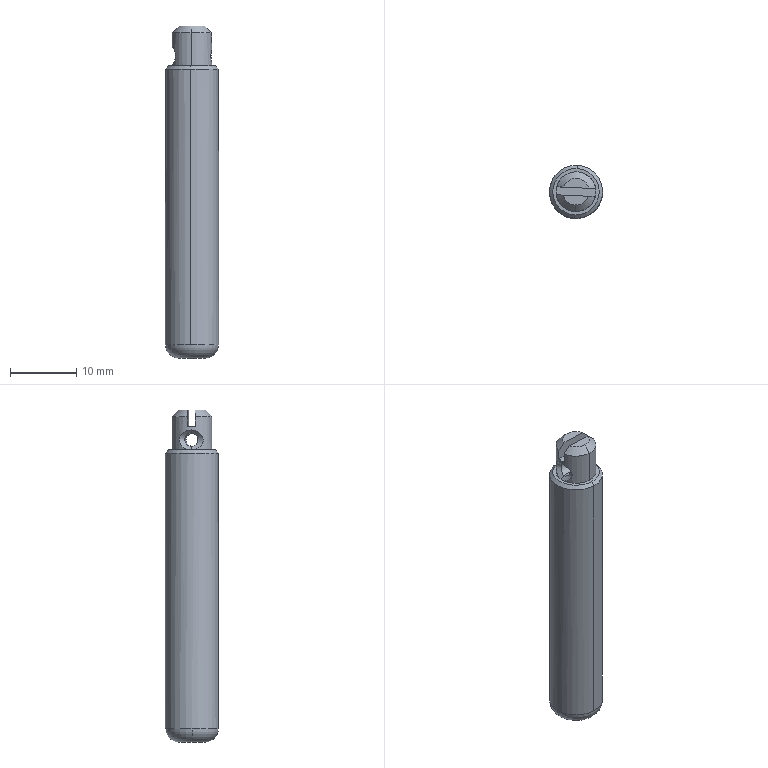Part | SolidWorks | features BaseBody 1 | 1 solid | 22 faces | box 8 x 8 x 50 mm | volume 2314 mm3 | plane 7 | cylinder 6 | cone 5 | spline 2 | torus 2 | commonest cylinder face diameters 2 x2 6 x2 8 x2
STEP:
#1=CARTESIAN_POINT('',(0.03983,28.012,-130.55));
#2=VERTEX_POINT('',#1);
#3=CARTESIAN_POINT('',(0.03996,28.015,-128.55));
#4=VERTEX_POINT('',#3);
#5=CARTESIAN_POINT('',(0.03983,28.012,-130.55));
#6=CARTESIAN_POINT('',(0.03364,27.875,-130.55));
#7=CARTESIAN_POINT('',(0.05576,27.735,-130.519));
#8=CARTESIAN_POINT('',(0.133,27.49,-130.414));
#9=CARTESIAN_POINT('',(0.187,27.383,-130.341));
#10=CARTESIAN_POINT('',(0.3031,27.204,-130.165));
#11=CARTESIAN_POINT('',(0.3627,27.129,-130.06));
#12=CARTESIAN_POINT('',(0.4571,27.024,-129.823));
#13=CARTESIAN_POINT('',(0.4923,26.992,-129.686));
#14=CARTESIAN_POINT('',(0.4912,26.993,-129.408));
#15=CARTESIAN_POINT('',(0.4562,27.025,-129.273));
#16=CARTESIAN_POINT('',(0.3609,27.132,-129.036));
#17=CARTESIAN_POINT('',(0.3014,27.205,-128.933));
#18=CARTESIAN_POINT('',(0.1856,27.386,-128.757));
#19=CARTESIAN_POINT('',(0.1323,27.492,-128.685));
#20=CARTESIAN_POINT('',(0.05554,27.737,-128.58));
#21=CARTESIAN_POINT('',(0.03327,27.875,-128.55));
#22=CARTESIAN_POINT('',(0.03996,28.015,-128.55));
#23=B_SPLINE_CURVE_WITH_KNOTS('',3,(#5,#6,#7,#8,#9,#10,#11,#12,#13,#14,#15,#16,#17,#18,#19,#20,#21,#22),.UNSPECIFIED.,.F.,.F.,(4,2,2,2,2,2,2,2,4),(0.003314,0.003727,0.00414,0.004553,0.004966,0.005379,0.005792,0.006205,0.006618),.UNSPECIFIED.);
#24=EDGE_CURVE('',#2,#4,#23,.T.);
#25=ORIENTED_EDGE('',*,*,#24,.F.);
#26=CARTESIAN_POINT('',(-0.4597,28.034,-131.05));
#27=VERTEX_POINT('',#26);
#28=CARTESIAN_POINT('',(0.03983,28.012,-130.55));
#29=CARTESIAN_POINT('',(-0.4597,28.034,-131.05));
#30=B_SPLINE_CURVE_WITH_KNOTS('',1,(#28,#29),.UNSPECIFIED.,.F.,.F.,(2,2),(0.009901,0.9896),.UNSPECIFIED.);
#31=EDGE_CURVE('',#2,#27,#30,.T.);
#32=ORIENTED_EDGE('',*,*,#31,.T.);
#33=CARTESIAN_POINT('',(-0.4595,28.039,-128.05));
#34=VERTEX_POINT('',#33);
#35=CARTESIAN_POINT('',(-0.4595,28.039,-128.05));
#36=CARTESIAN_POINT('',(-0.4701,27.815,-128.05));
#37=CARTESIAN_POINT('',(-0.4549,27.59,-128.084));
#38=CARTESIAN_POINT('',(-0.3813,27.169,-128.221));
#39=CARTESIAN_POINT('',(-0.3235,26.974,-128.322));
#40=CARTESIAN_POINT('',(-0.19,26.633,-128.58));
#41=CARTESIAN_POINT('',(-0.1141,26.487,-128.739));
#42=CARTESIAN_POINT('',(-0.02182,26.329,-129.02));
#43=CARTESIAN_POINT('',(0.005186,26.287,-129.121));
#44=CARTESIAN_POINT('',(0.0432,26.228,-129.331));
#45=CARTESIAN_POINT('',(0.05437,26.212,-129.443));
#46=CARTESIAN_POINT('',(0.05396,26.213,-129.664));
#47=CARTESIAN_POINT('',(0.04244,26.23,-129.775));
#48=CARTESIAN_POINT('',(0.003421,26.289,-129.986));
#49=CARTESIAN_POINT('',(-0.02341,26.332,-130.085));
#50=CARTESIAN_POINT('',(-0.1163,26.491,-130.366));
#51=CARTESIAN_POINT('',(-0.1903,26.633,-130.521));
#52=CARTESIAN_POINT('',(-0.3236,26.974,-130.778));
#53=CARTESIAN_POINT('',(-0.3805,27.166,-130.878));
#54=CARTESIAN_POINT('',(-0.4544,27.586,-131.015));
#55=CARTESIAN_POINT('',(-0.47,27.81,-131.05));
#56=CARTESIAN_POINT('',(-0.4597,28.034,-131.05));
#57=B_SPLINE_CURVE_WITH_KNOTS('',3,(#35,#36,#37,#38,#39,#40,#41,#42,#43,#44,#45,#46,#47,#48,#49,#50,#51,#52,#53,#54,#55,#56),.UNSPECIFIED.,.F.,.F.,(4,2,2,2,2,2,2,2,2,2,4),(0.005374,0.006046,0.006718,0.007391,0.007727,0.008063,0.008399,0.008735,0.009407,0.01008,0.01075),.UNSPECIFIED.);
#58=EDGE_CURVE('',#34,#27,#57,.T.);
#59=ORIENTED_EDGE('',*,*,#58,.F.);
#60=CARTESIAN_POINT('',(0.03996,28.015,-128.55));
#61=CARTESIAN_POINT('',(-0.4595,28.039,-128.05));
#62=B_SPLINE_CURVE_WITH_KNOTS('',1,(#60,#61),.UNSPECIFIED.,.F.,.F.,(2,2),(0.009901,0.9896),.UNSPECIFIED.);
#63=EDGE_CURVE('',#4,#34,#62,.T.);
#64=ORIENTED_EDGE('',*,*,#63,.F.);
#65=EDGE_LOOP('',(#25,#32,#59,#64));
#66=FACE_OUTER_BOUND('',#65,.T.);
#67=CARTESIAN_POINT('',(0.04501,28.015,-128.555));
#68=CARTESIAN_POINT('',(0.0577,28.283,-128.555));
#69=CARTESIAN_POINT('',(0.1783,28.533,-128.668));
#70=CARTESIAN_POINT('',(0.4502,28.877,-129.026));
#71=CARTESIAN_POINT('',(0.591,28.982,-129.281));
#72=CARTESIAN_POINT('',(0.5903,28.982,-129.822));
#73=CARTESIAN_POINT('',(0.4498,28.876,-130.075));
#74=CARTESIAN_POINT('',(0.1781,28.533,-130.432));
#75=CARTESIAN_POINT('',(0.05703,28.282,-130.546));
#76=CARTESIAN_POINT('',(0.03273,27.743,-130.544));
#77=CARTESIAN_POINT('',(0.1297,27.484,-130.43));
#78=CARTESIAN_POINT('',(0.3675,27.117,-130.072));
#79=CARTESIAN_POINT('',(0.4972,27.,-129.817));
#80=CARTESIAN_POINT('',(0.4952,27.001,-129.277));
#81=CARTESIAN_POINT('',(0.3667,27.119,-129.027));
#82=CARTESIAN_POINT('',(0.129,27.485,-128.669));
#83=CARTESIAN_POINT('',(0.03231,27.747,-128.555));
#84=CARTESIAN_POINT('',(0.04501,28.015,-128.555));
#85=CARTESIAN_POINT('',(-0.4595,28.039,-128.05));
#86=CARTESIAN_POINT('',(-0.4364,28.525,-128.05));
#87=CARTESIAN_POINT('',(-0.2839,28.983,-128.22));
#88=CARTESIAN_POINT('',(0.05333,29.613,-128.76));
#89=CARTESIAN_POINT('',(0.226,29.809,-129.144));
#90=CARTESIAN_POINT('',(0.225,29.808,-129.959));
#91=CARTESIAN_POINT('',(0.0529,29.613,-130.341));
#92=CARTESIAN_POINT('',(-0.2841,28.982,-130.88));
#93=CARTESIAN_POINT('',(-0.4372,28.523,-131.051));
#94=CARTESIAN_POINT('',(-0.4822,27.545,-131.049));
#95=CARTESIAN_POINT('',(-0.373,27.079,-130.877));
#96=CARTESIAN_POINT('',(-0.09732,26.421,-130.337));
#97=CARTESIAN_POINT('',(0.05533,26.211,-129.953));
#98=CARTESIAN_POINT('',(0.05298,26.214,-129.139));
#99=CARTESIAN_POINT('',(-0.09835,26.423,-128.761));
#100=CARTESIAN_POINT('',(-0.3738,27.081,-128.221));
#101=CARTESIAN_POINT('',(-0.4826,27.553,-128.05));
#102=CARTESIAN_POINT('',(-0.4595,28.039,-128.05));
#103=CARTESIAN_POINT('',(-0.4648,28.039,-128.045));
#104=CARTESIAN_POINT('',(-0.4416,28.528,-128.045));
#105=CARTESIAN_POINT('',(-0.2888,28.987,-128.216));
#106=CARTESIAN_POINT('',(0.04915,29.621,-128.757));
#107=CARTESIAN_POINT('',(0.2222,29.818,-129.143));
#108=CARTESIAN_POINT('',(0.2212,29.817,-129.961));
#109=CARTESIAN_POINT('',(0.04872,29.621,-130.344));
#110=CARTESIAN_POINT('',(-0.289,28.987,-130.885));
#111=CARTESIAN_POINT('',(-0.4425,28.525,-131.056));
#112=CARTESIAN_POINT('',(-0.4876,27.543,-131.054));
#113=CARTESIAN_POINT('',(-0.3783,27.074,-130.882));
#114=CARTESIAN_POINT('',(-0.1022,26.413,-130.34));
#115=CARTESIAN_POINT('',(0.05068,26.203,-129.954));
#116=CARTESIAN_POINT('',(0.04832,26.206,-129.138));
#117=CARTESIAN_POINT('',(-0.1033,26.416,-128.759));
#118=CARTESIAN_POINT('',(-0.3791,27.076,-128.216));
#119=CARTESIAN_POINT('',(-0.488,27.551,-128.045));
#120=CARTESIAN_POINT('',(-0.4648,28.039,-128.045));
#121=B_SPLINE_SURFACE_WITH_KNOTS('',1,3,((#67,#68,#69,#70,#71,#72,#73,#74,#75,#76,#77,#78,#79,#80,#81,#82,#83,#84),(#85,#86,#87,#88,#89,#90,#91,#92,#93,#94,#95,#96,#97,#98,#99,#100,#101,#102),(#103,#104,#105,#106,#107,#108,#109,#110,#111,#112,#113,#114,#115,#116,#117,#118,#119,#120)),.UNSPECIFIED.,.F.,.T.,.F.,(2,1,2),(4,2,2,2,2,2,2,2,4),(0.,0.9896,1.),(0.,0.125,0.25,0.375,0.5,0.625,0.75,0.875,1.),.UNSPECIFIED.);
#122=ADVANCED_FACE('',(#66),#121,.T.);
#123=CARTESIAN_POINT('',(2.347,23.901,-131.55));
#124=VERTEX_POINT('',#123);
#125=CARTESIAN_POINT('',(2.728,31.892,-131.55));
#126=VERTEX_POINT('',#125);
#127=CARTESIAN_POINT('',(2.537,27.896,-131.55));
#128=DIRECTION('',(0.,0.,-1.));
#129=DIRECTION('',(0.0476,0.9989,0.));
#130=AXIS2_PLACEMENT_3D('',#127,#128,#129);
#131=CIRCLE('',#130,4.);
#132=EDGE_CURVE('',#124,#126,#131,.T.);
#133=ORIENTED_EDGE('',*,*,#132,.T.);
#134=CARTESIAN_POINT('',(2.728,31.892,-173.05));
#135=VERTEX_POINT('',#134);
#136=CARTESIAN_POINT('',(2.728,31.892,-125.05));
#137=DIRECTION('',(0.,0.,-1.));
#138=VECTOR('',#137,1000.);
#139=LINE('',#136,#138);
#140=EDGE_CURVE('',#126,#135,#139,.T.);
#141=ORIENTED_EDGE('',*,*,#140,.T.);
#142=CARTESIAN_POINT('',(-1.463,27.896,-173.05));
#143=VERTEX_POINT('',#142);
#144=CARTESIAN_POINT('',(2.537,27.896,-173.05));
#145=DIRECTION('',(0.,0.,1.));
#146=DIRECTION('',(0.0476,0.9989,0.));
#147=AXIS2_PLACEMENT_3D('',#144,#145,#146);
#148=CIRCLE('',#147,4.);
#149=EDGE_CURVE('',#135,#143,#148,.T.);
#150=ORIENTED_EDGE('',*,*,#149,.T.);
#151=CARTESIAN_POINT('',(2.347,23.901,-173.05));
#152=VERTEX_POINT('',#151);
#153=CARTESIAN_POINT('',(2.537,27.896,-173.05));
#154=DIRECTION('',(0.,0.,1.));
#155=DIRECTION('',(0.0476,0.9989,0.));
#156=AXIS2_PLACEMENT_3D('',#153,#154,#155);
#157=CIRCLE('',#156,4.);
#158=EDGE_CURVE('',#143,#152,#157,.T.);
#159=ORIENTED_EDGE('',*,*,#158,.T.);
#160=CARTESIAN_POINT('',(2.347,23.901,-125.05));
#161=DIRECTION('',(0.,0.,-1.));
#162=VECTOR('',#161,1000.);
#163=LINE('',#160,#162);
#164=EDGE_CURVE('',#124,#152,#163,.T.);
#165=ORIENTED_EDGE('',*,*,#164,.F.);
#166=EDGE_LOOP('',(#133,#141,#150,#159,#165));
#167=FACE_OUTER_BOUND('',#166,.T.);
#168=CARTESIAN_POINT('',(2.537,27.896,-125.05));
#169=DIRECTION('',(0.,0.,-1.));
#170=DIRECTION('',(-0.0476,-0.9989,0.));
#171=AXIS2_PLACEMENT_3D('',#168,#169,#170);
#172=CYLINDRICAL_SURFACE('',#171,4.);
#173=ADVANCED_FACE('',(#167),#172,.T.);
#174=CARTESIAN_POINT('',(-0.4595,28.039,-131.05));
#175=VERTEX_POINT('',#174);
#176=CARTESIAN_POINT('',(2.394,24.9,-131.05));
#177=VERTEX_POINT('',#176);
#178=CARTESIAN_POINT('',(2.537,27.896,-131.05));
#179=DIRECTION('',(0.,0.,1.));
#180=DIRECTION('',(0.0476,0.9989,0.));
#181=AXIS2_PLACEMENT_3D('',#178,#179,#180);
#182=CIRCLE('',#181,3.);
#183=EDGE_CURVE('',#175,#177,#182,.T.);
#184=ORIENTED_EDGE('',*,*,#183,.T.);
#185=CARTESIAN_POINT('',(2.394,24.9,-126.05));
#186=VERTEX_POINT('',#185);
#187=CARTESIAN_POINT('',(2.394,24.9,-131.05));
#188=DIRECTION('',(0.,0.,1.));
#189=VECTOR('',#188,1000.);
#190=LINE('',#187,#189);
#191=EDGE_CURVE('',#177,#186,#190,.T.);
#192=ORIENTED_EDGE('',*,*,#191,.T.);
#193=CARTESIAN_POINT('',(-0.4275,27.437,-126.05));
#194=VERTEX_POINT('',#193);
#195=CARTESIAN_POINT('',(2.537,27.896,-126.05));
#196=DIRECTION('',(0.,0.,-1.));
#197=DIRECTION('',(0.0476,0.9989,0.));
#198=AXIS2_PLACEMENT_3D('',#195,#196,#197);
#199=CIRCLE('',#198,3.);
#200=EDGE_CURVE('',#186,#194,#199,.T.);
#201=ORIENTED_EDGE('',*,*,#200,.T.);
#202=CARTESIAN_POINT('',(-0.4275,27.437,-127.55));
#203=VERTEX_POINT('',#202);
#204=CARTESIAN_POINT('',(-0.4275,27.437,-127.55));
#205=DIRECTION('',(0.,0.,-1.));
#206=VECTOR('',#205,1000.);
#207=LINE('',#204,#206);
#208=EDGE_CURVE('',#194,#203,#207,.T.);
#209=ORIENTED_EDGE('',*,*,#208,.T.);
#210=CARTESIAN_POINT('',(-0.3704,28.635,-127.55));
#211=VERTEX_POINT('',#210);
#212=CARTESIAN_POINT('',(2.537,27.896,-127.55));
#213=DIRECTION('',(0.,0.,1.));
#214=DIRECTION('',(0.0476,0.9989,0.));
#215=AXIS2_PLACEMENT_3D('',#212,#213,#214);
#216=CIRCLE('',#215,3.);
#217=EDGE_CURVE('',#211,#203,#216,.T.);
#218=ORIENTED_EDGE('',*,*,#217,.F.);
#219=CARTESIAN_POINT('',(-0.3704,28.635,-126.05));
#220=VERTEX_POINT('',#219);
#221=CARTESIAN_POINT('',(-0.3704,28.635,-127.55));
#222=DIRECTION('',(0.,0.,-1.));
#223=VECTOR('',#222,1000.);
#224=LINE('',#221,#223);
#225=EDGE_CURVE('',#220,#211,#224,.T.);
#226=ORIENTED_EDGE('',*,*,#225,.F.);
#227=CARTESIAN_POINT('',(2.68,30.893,-126.05));
#228=VERTEX_POINT('',#227);
#229=CARTESIAN_POINT('',(2.537,27.896,-126.05));
#230=DIRECTION('',(0.,0.,-1.));
#231=DIRECTION('',(0.0476,0.9989,0.));
#232=AXIS2_PLACEMENT_3D('',#229,#230,#231);
#233=CIRCLE('',#232,3.);
#234=EDGE_CURVE('',#220,#228,#233,.T.);
#235=ORIENTED_EDGE('',*,*,#234,.T.);
#236=CARTESIAN_POINT('',(2.68,30.893,-131.05));
#237=VERTEX_POINT('',#236);
#238=CARTESIAN_POINT('',(2.68,30.893,-131.05));
#239=DIRECTION('',(0.,0.,1.));
#240=VECTOR('',#239,1000.);
#241=LINE('',#238,#240);
#242=EDGE_CURVE('',#237,#228,#241,.T.);
#243=ORIENTED_EDGE('',*,*,#242,.F.);
#244=CARTESIAN_POINT('',(2.537,27.896,-131.05));
#245=DIRECTION('',(0.,0.,1.));
#246=DIRECTION('',(0.0476,0.9989,0.));
#247=AXIS2_PLACEMENT_3D('',#244,#245,#246);
#248=CIRCLE('',#247,3.);
#249=EDGE_CURVE('',#237,#175,#248,.T.);
#250=ORIENTED_EDGE('',*,*,#249,.T.);
#251=CARTESIAN_POINT('',(-0.4595,28.039,-131.05));
#252=CARTESIAN_POINT('',(-0.4488,28.263,-131.05));
#253=CARTESIAN_POINT('',(-0.4123,28.485,-131.016));
#254=CARTESIAN_POINT('',(-0.2992,28.896,-130.879));
#255=CARTESIAN_POINT('',(-0.2232,29.085,-130.778));
#256=CARTESIAN_POINT('',(-0.05789,29.413,-130.521));
#257=CARTESIAN_POINT('',(0.03136,29.55,-130.362));
#258=CARTESIAN_POINT('',(0.1384,29.699,-130.081));
#259=CARTESIAN_POINT('',(0.1692,29.738,-129.981));
#260=CARTESIAN_POINT('',(0.2128,29.793,-129.771));
#261=CARTESIAN_POINT('',(0.2257,29.809,-129.659));
#262=CARTESIAN_POINT('',(0.2254,29.808,-129.437));
#263=CARTESIAN_POINT('',(0.2122,29.793,-129.325));
#264=CARTESIAN_POINT('',(0.1677,29.737,-129.115));
#265=CARTESIAN_POINT('',(0.1363,29.696,-129.014));
#266=CARTESIAN_POINT('',(0.02984,29.548,-128.736));
#267=CARTESIAN_POINT('',(-0.05896,29.411,-128.577));
#268=CARTESIAN_POINT('',(-0.2241,29.083,-128.32));
#269=CARTESIAN_POINT('',(-0.2992,28.897,-128.221));
#270=CARTESIAN_POINT('',(-0.4122,28.485,-128.084));
#271=CARTESIAN_POINT('',(-0.4488,28.263,-128.05));
#272=CARTESIAN_POINT('',(-0.4595,28.039,-128.05));
#273=B_SPLINE_CURVE_WITH_KNOTS('',3,(#251,#252,#253,#254,#255,#256,#257,#258,#259,#260,#261,#262,#263,#264,#265,#266,#267,#268,#269,#270,#271,#272),.UNSPECIFIED.,.F.,.F.,(4,2,2,2,2,2,2,2,2,2,4),(0.,0.0006718,0.001344,0.002015,0.002351,0.002687,0.003023,0.003359,0.004031,0.004702,0.005374),.UNSPECIFIED.);
#274=EDGE_CURVE('',#175,#34,#273,.T.);
#275=ORIENTED_EDGE('',*,*,#274,.T.);
#276=ORIENTED_EDGE('',*,*,#58,.T.);
#277=CARTESIAN_POINT('',(-0.4597,28.034,-131.05));
#278=CARTESIAN_POINT('',(-0.4597,28.035,-131.05));
#279=CARTESIAN_POINT('',(-0.4596,28.036,-131.05));
#280=CARTESIAN_POINT('',(-0.4596,28.037,-131.05));
#281=CARTESIAN_POINT('',(-0.4595,28.038,-131.05));
#282=CARTESIAN_POINT('',(-0.4595,28.039,-131.05));
#283=B_SPLINE_CURVE_WITH_KNOTS('',3,(#277,#278,#279,#280,#281,#282),.UNSPECIFIED.,.F.,.F.,(4,2,4),(0.01075,0.01075,0.01076),.UNSPECIFIED.);
#284=EDGE_CURVE('',#27,#175,#283,.T.);
#285=ORIENTED_EDGE('',*,*,#284,.T.);
#286=EDGE_LOOP('',(#184,#192,#201,#209,#218,#226,#235,#243,#250,#275,#276,#285));
#287=FACE_OUTER_BOUND('',#286,.T.);
#288=CARTESIAN_POINT('',(2.537,27.896,-131.05));
#289=DIRECTION('',(0.,0.,1.));
#290=DIRECTION('',(0.0476,0.9989,0.));
#291=AXIS2_PLACEMENT_3D('',#288,#289,#290);
#292=CYLINDRICAL_SURFACE('',#291,3.);
#293=ADVANCED_FACE('',(#287),#292,.T.);
#294=CARTESIAN_POINT('',(5.534,27.753,-128.55));
#295=VERTEX_POINT('',#294);
#296=CARTESIAN_POINT('',(5.534,27.753,-130.55));
#297=VERTEX_POINT('',#296);
#298=CARTESIAN_POINT('',(5.534,27.753,-128.55));
#299=CARTESIAN_POINT('',(5.527,27.62,-128.55));
#300=CARTESIAN_POINT('',(5.512,27.49,-128.577));
#301=CARTESIAN_POINT('',(5.469,27.25,-128.677));
#302=CARTESIAN_POINT('',(5.442,27.141,-128.751));
#303=CARTESIAN_POINT('',(5.389,26.961,-128.935));
#304=CARTESIAN_POINT('',(5.363,26.887,-129.045));
#305=CARTESIAN_POINT('',(5.326,26.789,-129.286));
#306=CARTESIAN_POINT('',(5.315,26.763,-129.418));
#307=CARTESIAN_POINT('',(5.315,26.763,-129.682));
#308=CARTESIAN_POINT('',(5.326,26.788,-129.813));
#309=CARTESIAN_POINT('',(5.363,26.888,-130.056));
#310=CARTESIAN_POINT('',(5.389,26.96,-130.165));
#311=CARTESIAN_POINT('',(5.442,27.142,-130.349));
#312=CARTESIAN_POINT('',(5.469,27.251,-130.423));
#313=CARTESIAN_POINT('',(5.512,27.491,-130.523));
#314=CARTESIAN_POINT('',(5.527,27.622,-130.55));
#315=CARTESIAN_POINT('',(5.534,27.753,-130.55));
#316=B_SPLINE_CURVE_WITH_KNOTS('',3,(#298,#299,#300,#301,#302,#303,#304,#305,#306,#307,#308,#309,#310,#311,#312,#313,#314,#315),.UNSPECIFIED.,.F.,.F.,(4,2,2,2,2,2,2,2,4),(0.,0.0003936,0.0007871,0.001181,0.001574,0.001968,0.002361,0.002755,0.003149),.UNSPECIFIED.);
#317=EDGE_CURVE('',#295,#297,#316,.T.);
#318=ORIENTED_EDGE('',*,*,#317,.T.);
#319=CARTESIAN_POINT('',(0.03996,28.015,-130.55));
#320=VERTEX_POINT('',#319);
#321=CARTESIAN_POINT('',(10.528,27.515,-130.55));
#322=DIRECTION('',(-0.9989,0.0476,0.));
#323=VECTOR('',#322,1000.);
#324=LINE('',#321,#323);
#325=EDGE_CURVE('',#297,#320,#324,.T.);
#326=ORIENTED_EDGE('',*,*,#325,.T.);
#327=CARTESIAN_POINT('',(0.03996,28.015,-130.55));
#328=CARTESIAN_POINT('',(0.03994,28.015,-130.55));
#329=CARTESIAN_POINT('',(0.03989,28.014,-130.55));
#330=CARTESIAN_POINT('',(0.03985,28.013,-130.55));
#331=CARTESIAN_POINT('',(0.03983,28.012,-130.55));
#332=B_SPLINE_CURVE_WITH_KNOTS('',3,(#327,#328,#329,#330,#331),.UNSPECIFIED.,.F.,.F.,(4,1,4),(0.003311,0.003313,0.003314),.UNSPECIFIED.);
#333=EDGE_CURVE('',#320,#2,#332,.T.);
#334=ORIENTED_EDGE('',*,*,#333,.T.);
#335=ORIENTED_EDGE('',*,*,#24,.T.);
#336=CARTESIAN_POINT('',(10.528,27.515,-128.55));
#337=DIRECTION('',(-0.9989,0.0476,0.));
#338=VECTOR('',#337,1000.);
#339=LINE('',#336,#338);
#340=EDGE_CURVE('',#295,#4,#339,.T.);
#341=ORIENTED_EDGE('',*,*,#340,.F.);
#342=EDGE_LOOP('',(#318,#326,#334,#335,#341));
#343=FACE_OUTER_BOUND('',#342,.T.);
#344=CARTESIAN_POINT('',(10.528,27.515,-129.55));
#345=DIRECTION('',(-0.9989,0.0476,0.));
#346=DIRECTION('',(0.,0.,1.));
#347=AXIS2_PLACEMENT_3D('',#344,#345,#346);
#348=CYLINDRICAL_SURFACE('',#347,1.);
#349=ADVANCED_FACE('',(#343),#348,.F.);
#350=CARTESIAN_POINT('',(2.442,25.898,-125.05));
#351=VERTEX_POINT('',#350);
#352=CARTESIAN_POINT('',(4.414,27.206,-125.05));
#353=VERTEX_POINT('',#352);
#354=CARTESIAN_POINT('',(2.537,27.896,-125.05));
#355=DIRECTION('',(0.,0.,1.));
#356=DIRECTION('',(0.0476,0.9989,0.));
#357=AXIS2_PLACEMENT_3D('',#354,#355,#356);
#358=CIRCLE('',#357,2.);
#359=EDGE_CURVE('',#351,#353,#358,.T.);
#360=ORIENTED_EDGE('',*,*,#359,.F.);
#361=CARTESIAN_POINT('',(2.442,25.898,-125.05));
#362=DIRECTION('',(-0.03366,-0.7063,-0.7071));
#363=VECTOR('',#362,1000.);
#364=LINE('',#361,#363);
#365=EDGE_CURVE('',#351,#186,#364,.T.);
#366=ORIENTED_EDGE('',*,*,#365,.T.);
#367=CARTESIAN_POINT('',(5.445,27.157,-126.05));
#368=VERTEX_POINT('',#367);
#369=CARTESIAN_POINT('',(2.537,27.896,-126.05));
#370=DIRECTION('',(0.,0.,-1.));
#371=DIRECTION('',(0.0476,0.9989,0.));
#372=AXIS2_PLACEMENT_3D('',#369,#370,#371);
#373=CIRCLE('',#372,3.);
#374=EDGE_CURVE('',#368,#186,#373,.T.);
#375=ORIENTED_EDGE('',*,*,#374,.F.);
#376=CARTESIAN_POINT('',(4.414,27.206,-125.05));
#377=CARTESIAN_POINT('',(4.76,27.19,-125.381));
#378=CARTESIAN_POINT('',(5.103,27.173,-125.715));
#379=CARTESIAN_POINT('',(5.445,27.157,-126.05));
#380=B_SPLINE_CURVE_WITH_KNOTS('',3,(#376,#377,#378,#379),.UNSPECIFIED.,.F.,.F.,(4,4),(0.,0.001437),.UNSPECIFIED.);
#381=EDGE_CURVE('',#353,#368,#380,.T.);
#382=ORIENTED_EDGE('',*,*,#381,.F.);
#383=EDGE_LOOP('',(#360,#366,#375,#382));
#384=FACE_OUTER_BOUND('',#383,.T.);
#385=CARTESIAN_POINT('',(2.537,27.896,-125.05));
#386=DIRECTION('',(0.,0.,-1.));
#387=DIRECTION('',(-0.0476,-0.9989,0.));
#388=AXIS2_PLACEMENT_3D('',#385,#386,#387);
#389=CONICAL_SURFACE('',#388,2.,0.7854);
#390=ADVANCED_FACE('',(#384),#389,.T.);
#391=CARTESIAN_POINT('',(2.704,31.392,-131.05));
#392=VERTEX_POINT('',#391);
#393=CARTESIAN_POINT('',(2.371,24.4,-131.05));
#394=VERTEX_POINT('',#393);
#395=CARTESIAN_POINT('',(2.537,27.896,-131.05));
#396=DIRECTION('',(0.,0.,1.));
#397=DIRECTION('',(0.0476,0.9989,0.));
#398=AXIS2_PLACEMENT_3D('',#395,#396,#397);
#399=CIRCLE('',#398,3.5);
#400=EDGE_CURVE('',#392,#394,#399,.T.);
#401=ORIENTED_EDGE('',*,*,#400,.F.);
#402=CARTESIAN_POINT('',(2.704,31.392,-131.05));
#403=DIRECTION('',(0.03366,0.7063,-0.7071));
#404=VECTOR('',#403,1000.);
#405=LINE('',#402,#404);
#406=EDGE_CURVE('',#392,#126,#405,.T.);
#407=ORIENTED_EDGE('',*,*,#406,.T.);
#408=ORIENTED_EDGE('',*,*,#132,.F.);
#409=CARTESIAN_POINT('',(2.371,24.4,-131.05));
#410=DIRECTION('',(-0.03366,-0.7063,-0.7071));
#411=VECTOR('',#410,1000.);
#412=LINE('',#409,#411);
#413=EDGE_CURVE('',#394,#124,#412,.T.);
#414=ORIENTED_EDGE('',*,*,#413,.F.);
#415=EDGE_LOOP('',(#401,#407,#408,#414));
#416=FACE_OUTER_BOUND('',#415,.T.);
#417=CARTESIAN_POINT('',(2.537,27.896,-131.05));
#418=DIRECTION('',(0.,0.,-1.));
#419=DIRECTION('',(-0.0476,-0.9989,0.));
#420=AXIS2_PLACEMENT_3D('',#417,#418,#419);
#421=CONICAL_SURFACE('',#420,3.5,0.7854);
#422=ADVANCED_FACE('',(#416),#421,.T.);
#423=CARTESIAN_POINT('',(4.537,27.896,-175.05));
#424=VERTEX_POINT('',#423);
#425=CARTESIAN_POINT('',(0.5371,27.896,-175.05));
#426=VERTEX_POINT('',#425);
#427=CARTESIAN_POINT('',(2.537,27.896,-175.05));
#428=DIRECTION('',(0.,0.,-1.));
#429=DIRECTION('',(0.0476,0.9989,0.));
#430=AXIS2_PLACEMENT_3D('',#427,#428,#429);
#431=CIRCLE('',#430,2.);
#432=EDGE_CURVE('',#424,#426,#431,.T.);
#433=ORIENTED_EDGE('',*,*,#432,.F.);
#434=CARTESIAN_POINT('',(6.537,27.896,-173.05));
#435=VERTEX_POINT('',#434);
#436=CARTESIAN_POINT('',(4.537,27.896,-173.05));
#437=DIRECTION('',(0.,-1.,0.));
#438=DIRECTION('',(1.,0.,0.));
#439=AXIS2_PLACEMENT_3D('',#436,#437,#438);
#440=CIRCLE('',#439,2.);
#441=EDGE_CURVE('',#424,#435,#440,.T.);
#442=ORIENTED_EDGE('',*,*,#441,.T.);
#443=CARTESIAN_POINT('',(2.537,27.896,-173.05));
#444=DIRECTION('',(0.,0.,1.));
#445=DIRECTION('',(0.0476,0.9989,0.));
#446=AXIS2_PLACEMENT_3D('',#443,#444,#445);
#447=CIRCLE('',#446,4.);
#448=EDGE_CURVE('',#152,#435,#447,.T.);
#449=ORIENTED_EDGE('',*,*,#448,.F.);
#450=ORIENTED_EDGE('',*,*,#158,.F.);
#451=CARTESIAN_POINT('',(0.5371,27.896,-173.05));
#452=DIRECTION('',(0.,1.,0.));
#453=DIRECTION('',(0.,0.,1.));
#454=AXIS2_PLACEMENT_3D('',#451,#452,#453);
#455=CIRCLE('',#454,2.);
#456=EDGE_CURVE('',#426,#143,#455,.T.);
#457=ORIENTED_EDGE('',*,*,#456,.F.);
#458=EDGE_LOOP('',(#433,#442,#449,#450,#457));
#459=FACE_OUTER_BOUND('',#458,.T.);
#460=CARTESIAN_POINT('',(2.537,27.896,-173.05));
#461=DIRECTION('',(0.,0.,1.));
#462=DIRECTION('',(-1.,0.,0.));
#463=AXIS2_PLACEMENT_3D('',#460,#461,#462);
#464=TOROIDAL_SURFACE('',#463,2.,2.);
#465=ADVANCED_FACE('',(#459),#464,.T.);
#466=ORIENTED_EDGE('',*,*,#441,.F.);
#467=CARTESIAN_POINT('',(2.537,27.896,-175.05));
#468=DIRECTION('',(0.,0.,-1.));
#469=DIRECTION('',(0.0476,0.9989,0.));
#470=AXIS2_PLACEMENT_3D('',#467,#468,#469);
#471=CIRCLE('',#470,2.);
#472=EDGE_CURVE('',#426,#424,#471,.T.);
#473=ORIENTED_EDGE('',*,*,#472,.F.);
#474=ORIENTED_EDGE('',*,*,#456,.T.);
#475=ORIENTED_EDGE('',*,*,#149,.F.);
#476=CARTESIAN_POINT('',(2.537,27.896,-173.05));
#477=DIRECTION('',(0.,0.,1.));
#478=DIRECTION('',(0.0476,0.9989,0.));
#479=AXIS2_PLACEMENT_3D('',#476,#477,#478);
#480=CIRCLE('',#479,4.);
#481=EDGE_CURVE('',#435,#135,#480,.T.);
#482=ORIENTED_EDGE('',*,*,#481,.F.);
#483=EDGE_LOOP('',(#466,#473,#474,#475,#482));
#484=FACE_OUTER_BOUND('',#483,.T.);
#485=CARTESIAN_POINT('',(2.537,27.896,-173.05));
#486=DIRECTION('',(0.,0.,1.));
#487=DIRECTION('',(-1.,0.,0.));
#488=AXIS2_PLACEMENT_3D('',#485,#486,#487);
#489=TOROIDAL_SURFACE('',#488,2.,2.);
#490=ADVANCED_FACE('',(#484),#489,.T.);
#491=ORIENTED_EDGE('',*,*,#406,.F.);
#492=CARTESIAN_POINT('',(2.537,27.896,-131.05));
#493=DIRECTION('',(0.,0.,1.));
#494=DIRECTION('',(0.0476,0.9989,0.));
#495=AXIS2_PLACEMENT_3D('',#492,#493,#494);
#496=CIRCLE('',#495,3.5);
#497=EDGE_CURVE('',#394,#392,#496,.T.);
#498=ORIENTED_EDGE('',*,*,#497,.F.);
#499=ORIENTED_EDGE('',*,*,#413,.T.);
#500=CARTESIAN_POINT('',(2.537,27.896,-131.55));
#501=DIRECTION('',(0.,0.,-1.));
#502=DIRECTION('',(0.0476,0.9989,0.));
#503=AXIS2_PLACEMENT_3D('',#500,#501,#502);
#504=CIRCLE('',#503,4.);
#505=EDGE_CURVE('',#126,#124,#504,.T.);
#506=ORIENTED_EDGE('',*,*,#505,.F.);
#507=EDGE_LOOP('',(#491,#498,#499,#506));
#508=FACE_OUTER_BOUND('',#507,.T.);
#509=CARTESIAN_POINT('',(2.537,27.896,-131.05));
#510=DIRECTION('',(0.,0.,-1.));
#511=DIRECTION('',(-0.0476,-0.9989,0.));
#512=AXIS2_PLACEMENT_3D('',#509,#510,#511);
#513=CONICAL_SURFACE('',#512,3.5,0.7854);
#514=ADVANCED_FACE('',(#508),#513,.T.);
#515=ORIENTED_EDGE('',*,*,#365,.F.);
#516=CARTESIAN_POINT('',(0.6028,27.388,-125.05));
#517=VERTEX_POINT('',#516);
#518=CARTESIAN_POINT('',(2.537,27.896,-125.05));
#519=DIRECTION('',(0.,0.,1.));
#520=DIRECTION('',(0.0476,0.9989,0.));
#521=AXIS2_PLACEMENT_3D('',#518,#519,#520);
#522=CIRCLE('',#521,2.);
#523=EDGE_CURVE('',#517,#351,#522,.T.);
#524=ORIENTED_EDGE('',*,*,#523,.F.);
#525=CARTESIAN_POINT('',(-0.4275,27.437,-126.05));
#526=CARTESIAN_POINT('',(-0.08581,27.421,-125.715));
#527=CARTESIAN_POINT('',(0.2567,27.404,-125.381));
#528=CARTESIAN_POINT('',(0.6028,27.388,-125.05));
#529=B_SPLINE_CURVE_WITH_KNOTS('',3,(#525,#526,#527,#528),.UNSPECIFIED.,.F.,.F.,(4,4),(0.,0.001437),.UNSPECIFIED.);
#530=EDGE_CURVE('',#194,#517,#529,.T.);
#531=ORIENTED_EDGE('',*,*,#530,.F.);
#532=ORIENTED_EDGE('',*,*,#200,.F.);
#533=EDGE_LOOP('',(#515,#524,#531,#532));
#534=FACE_OUTER_BOUND('',#533,.T.);
#535=CARTESIAN_POINT('',(2.537,27.896,-125.05));
#536=DIRECTION('',(0.,0.,-1.));
#537=DIRECTION('',(-0.0476,-0.9989,0.));
#538=AXIS2_PLACEMENT_3D('',#535,#536,#537);
#539=CONICAL_SURFACE('',#538,2.,0.7854);
#540=ADVANCED_FACE('',(#534),#539,.T.);
#541=CARTESIAN_POINT('',(5.502,28.356,-126.05));
#542=VERTEX_POINT('',#541);
#543=CARTESIAN_POINT('',(4.471,28.405,-125.05));
#544=VERTEX_POINT('',#543);
#545=CARTESIAN_POINT('',(5.502,28.356,-126.05));
#546=CARTESIAN_POINT('',(5.16,28.372,-125.715));
#547=CARTESIAN_POINT('',(4.818,28.388,-125.381));
#548=CARTESIAN_POINT('',(4.471,28.405,-125.05));
#549=B_SPLINE_CURVE_WITH_KNOTS('',3,(#545,#546,#547,#548),.UNSPECIFIED.,.F.,.F.,(4,4),(0.,0.001437),.UNSPECIFIED.);
#550=EDGE_CURVE('',#542,#544,#549,.T.);
#551=ORIENTED_EDGE('',*,*,#550,.F.);
#552=CARTESIAN_POINT('',(2.537,27.896,-126.05));
#553=DIRECTION('',(0.,0.,-1.));
#554=DIRECTION('',(0.0476,0.9989,0.));
#555=AXIS2_PLACEMENT_3D('',#552,#553,#554);
#556=CIRCLE('',#555,3.);
#557=EDGE_CURVE('',#228,#542,#556,.T.);
#558=ORIENTED_EDGE('',*,*,#557,.F.);
#559=ORIENTED_EDGE('',*,*,#234,.F.);
#560=CARTESIAN_POINT('',(0.66,28.586,-125.05));
#561=VERTEX_POINT('',#560);
#562=CARTESIAN_POINT('',(0.66,28.586,-125.05));
#563=CARTESIAN_POINT('',(0.3138,28.603,-125.381));
#564=CARTESIAN_POINT('',(-0.02869,28.619,-125.715));
#565=CARTESIAN_POINT('',(-0.3704,28.635,-126.05));
#566=B_SPLINE_CURVE_WITH_KNOTS('',3,(#562,#563,#564,#565),.UNSPECIFIED.,.F.,.F.,(4,4),(0.,0.001437),.UNSPECIFIED.);
#567=EDGE_CURVE('',#561,#220,#566,.T.);
#568=ORIENTED_EDGE('',*,*,#567,.F.);
#569=CARTESIAN_POINT('',(2.537,27.896,-125.05));
#570=DIRECTION('',(0.,0.,1.));
#571=DIRECTION('',(0.0476,0.9989,0.));
#572=AXIS2_PLACEMENT_3D('',#569,#570,#571);
#573=CIRCLE('',#572,2.);
#574=EDGE_CURVE('',#544,#561,#573,.T.);
#575=ORIENTED_EDGE('',*,*,#574,.F.);
#576=EDGE_LOOP('',(#551,#558,#559,#568,#575));
#577=FACE_OUTER_BOUND('',#576,.T.);
#578=CARTESIAN_POINT('',(2.537,27.896,-125.05));
#579=DIRECTION('',(0.,0.,-1.));
#580=DIRECTION('',(-0.0476,-0.9989,0.));
#581=AXIS2_PLACEMENT_3D('',#578,#579,#580);
#582=CONICAL_SURFACE('',#581,2.,0.7854);
#583=ADVANCED_FACE('',(#577),#582,.T.);
#584=CARTESIAN_POINT('',(5.445,27.157,-127.55));
#585=VERTEX_POINT('',#584);
#586=CARTESIAN_POINT('',(5.502,28.356,-127.55));
#587=VERTEX_POINT('',#586);
#588=CARTESIAN_POINT('',(2.537,27.896,-127.55));
#589=DIRECTION('',(0.,0.,1.));
#590=DIRECTION('',(0.0476,0.9989,0.));
#591=AXIS2_PLACEMENT_3D('',#588,#589,#590);
#592=CIRCLE('',#591,3.);
#593=EDGE_CURVE('',#585,#587,#592,.T.);
#594=ORIENTED_EDGE('',*,*,#593,.T.);
#595=CARTESIAN_POINT('',(-0.3704,28.635,-127.55));
#596=DIRECTION('',(-0.9989,0.0476,0.));
#597=VECTOR('',#596,1000.);
#598=LINE('',#595,#597);
#599=EDGE_CURVE('',#587,#211,#598,.T.);
#600=ORIENTED_EDGE('',*,*,#599,.T.);
#601=ORIENTED_EDGE('',*,*,#217,.T.);
#602=CARTESIAN_POINT('',(-0.4275,27.437,-127.55));
#603=DIRECTION('',(0.9989,-0.0476,0.));
#604=VECTOR('',#603,1000.);
#605=LINE('',#602,#604);
#606=EDGE_CURVE('',#203,#585,#605,.T.);
#607=ORIENTED_EDGE('',*,*,#606,.T.);
#608=EDGE_LOOP('',(#594,#600,#601,#607));
#609=FACE_OUTER_BOUND('',#608,.T.);
#610=CARTESIAN_POINT('',(2.537,27.896,-127.55));
#611=DIRECTION('',(0.,0.,1.));
#612=DIRECTION('',(1.,0.,0.));
#613=AXIS2_PLACEMENT_3D('',#610,#611,#612);
#614=PLANE('',#613);
#615=ADVANCED_FACE('',(#609),#614,.T.);
#616=CARTESIAN_POINT('',(-0.3704,28.635,-125.05));
#617=DIRECTION('',(-0.9989,0.0476,0.));
#618=VECTOR('',#617,1000.);
#619=LINE('',#616,#618);
#620=EDGE_CURVE('',#544,#561,#619,.T.);
#621=ORIENTED_EDGE('',*,*,#620,.T.);
#622=ORIENTED_EDGE('',*,*,#567,.T.);
#623=ORIENTED_EDGE('',*,*,#225,.T.);
#624=ORIENTED_EDGE('',*,*,#599,.F.);
#625=CARTESIAN_POINT('',(5.502,28.356,-127.55));
#626=DIRECTION('',(0.,0.,1.));
#627=VECTOR('',#626,1000.);
#628=LINE('',#625,#627);
#629=EDGE_CURVE('',#587,#542,#628,.T.);
#630=ORIENTED_EDGE('',*,*,#629,.T.);
#631=ORIENTED_EDGE('',*,*,#550,.T.);
#632=EDGE_LOOP('',(#621,#622,#623,#624,#630,#631));
#633=FACE_OUTER_BOUND('',#632,.T.);
#634=CARTESIAN_POINT('',(-0.3704,28.635,-127.55));
#635=DIRECTION('',(0.0476,0.9989,0.));
#636=DIRECTION('',(0.,0.,-1.));
#637=AXIS2_PLACEMENT_3D('',#634,#635,#636);
#638=PLANE('',#637);
#639=ADVANCED_FACE('',(#633),#638,.F.);
#640=CARTESIAN_POINT('',(-0.4275,27.437,-125.05));
#641=DIRECTION('',(0.9989,-0.0476,0.));
#642=VECTOR('',#641,1000.);
#643=LINE('',#640,#642);
#644=EDGE_CURVE('',#517,#353,#643,.T.);
#645=ORIENTED_EDGE('',*,*,#644,.T.);
#646=ORIENTED_EDGE('',*,*,#381,.T.);
#647=CARTESIAN_POINT('',(5.445,27.157,-127.55));
#648=DIRECTION('',(0.,0.,1.));
#649=VECTOR('',#648,1000.);
#650=LINE('',#647,#649);
#651=EDGE_CURVE('',#585,#368,#650,.T.);
#652=ORIENTED_EDGE('',*,*,#651,.F.);
#653=ORIENTED_EDGE('',*,*,#606,.F.);
#654=ORIENTED_EDGE('',*,*,#208,.F.);
#655=ORIENTED_EDGE('',*,*,#530,.T.);
#656=EDGE_LOOP('',(#645,#646,#652,#653,#654,#655));
#657=FACE_OUTER_BOUND('',#656,.T.);
#658=CARTESIAN_POINT('',(-0.4275,27.437,-127.55));
#659=DIRECTION('',(-0.0476,-0.9989,0.));
#660=DIRECTION('',(-0.9989,0.0476,0.));
#661=AXIS2_PLACEMENT_3D('',#658,#659,#660);
#662=PLANE('',#661);
#663=ADVANCED_FACE('',(#657),#662,.F.);
#664=ORIENTED_EDGE('',*,*,#31,.F.);
#665=ORIENTED_EDGE('',*,*,#333,.F.);
#666=CARTESIAN_POINT('',(0.03996,28.015,-128.55));
#667=CARTESIAN_POINT('',(0.04666,28.155,-128.55));
#668=CARTESIAN_POINT('',(0.08168,28.29,-128.58));
#669=CARTESIAN_POINT('',(0.1812,28.527,-128.684));
#670=CARTESIAN_POINT('',(0.2454,28.629,-128.758));
#671=CARTESIAN_POINT('',(0.3777,28.797,-128.933));
#672=CARTESIAN_POINT('',(0.4439,28.865,-129.037));
#673=CARTESIAN_POINT('',(0.5483,28.962,-129.274));
#674=CARTESIAN_POINT('',(0.587,28.99,-129.412));
#675=CARTESIAN_POINT('',(0.587,28.99,-129.689));
#676=CARTESIAN_POINT('',(0.5493,28.962,-129.825));
#677=CARTESIAN_POINT('',(0.4439,28.865,-130.063));
#678=CARTESIAN_POINT('',(0.3782,28.797,-130.166));
#679=CARTESIAN_POINT('',(0.2446,28.628,-130.343));
#680=CARTESIAN_POINT('',(0.1817,28.528,-130.415));
#681=CARTESIAN_POINT('',(0.1063,28.349,-130.494));
#682=CARTESIAN_POINT('',(0.08523,28.286,-130.515));
#683=CARTESIAN_POINT('',(0.05356,28.154,-130.543));
#684=CARTESIAN_POINT('',(0.04324,28.084,-130.55));
#685=CARTESIAN_POINT('',(0.03996,28.015,-130.55));
#686=B_SPLINE_CURVE_WITH_KNOTS('',3,(#666,#667,#668,#669,#670,#671,#672,#673,#674,#675,#676,#677,#678,#679,#680,#681,#682,#683,#684,#685),.UNSPECIFIED.,.F.,.F.,(4,2,2,2,2,2,2,2,2,4),(0.,0.0004139,0.0008278,0.001242,0.001656,0.002069,0.002483,0.002897,0.003104,0.003311),.UNSPECIFIED.);
#687=EDGE_CURVE('',#4,#320,#686,.T.);
#688=ORIENTED_EDGE('',*,*,#687,.F.);
#689=ORIENTED_EDGE('',*,*,#63,.T.);
#690=ORIENTED_EDGE('',*,*,#274,.F.);
#691=ORIENTED_EDGE('',*,*,#284,.F.);
#692=EDGE_LOOP('',(#664,#665,#688,#689,#690,#691));
#693=FACE_OUTER_BOUND('',#692,.T.);
#694=CARTESIAN_POINT('',(0.04501,28.015,-128.555));
#695=CARTESIAN_POINT('',(0.0577,28.283,-128.555));
#696=CARTESIAN_POINT('',(0.1783,28.533,-128.668));
#697=CARTESIAN_POINT('',(0.4502,28.877,-129.026));
#698=CARTESIAN_POINT('',(0.591,28.982,-129.281));
#699=CARTESIAN_POINT('',(0.5903,28.982,-129.822));
#700=CARTESIAN_POINT('',(0.4498,28.876,-130.075));
#701=CARTESIAN_POINT('',(0.1781,28.533,-130.432));
#702=CARTESIAN_POINT('',(0.05703,28.282,-130.546));
#703=CARTESIAN_POINT('',(0.03273,27.743,-130.544));
#704=CARTESIAN_POINT('',(0.1297,27.484,-130.43));
#705=CARTESIAN_POINT('',(0.3675,27.117,-130.072));
#706=CARTESIAN_POINT('',(0.4972,27.,-129.817));
#707=CARTESIAN_POINT('',(0.4952,27.001,-129.277));
#708=CARTESIAN_POINT('',(0.3667,27.119,-129.027));
#709=CARTESIAN_POINT('',(0.129,27.485,-128.669));
#710=CARTESIAN_POINT('',(0.03231,27.747,-128.555));
#711=CARTESIAN_POINT('',(0.04501,28.015,-128.555));
#712=CARTESIAN_POINT('',(-0.4595,28.039,-128.05));
#713=CARTESIAN_POINT('',(-0.4364,28.525,-128.05));
#714=CARTESIAN_POINT('',(-0.2839,28.983,-128.22));
#715=CARTESIAN_POINT('',(0.05333,29.613,-128.76));
#716=CARTESIAN_POINT('',(0.226,29.809,-129.144));
#717=CARTESIAN_POINT('',(0.225,29.808,-129.959));
#718=CARTESIAN_POINT('',(0.0529,29.613,-130.341));
#719=CARTESIAN_POINT('',(-0.2841,28.982,-130.88));
#720=CARTESIAN_POINT('',(-0.4372,28.523,-131.051));
#721=CARTESIAN_POINT('',(-0.4822,27.545,-131.049));
#722=CARTESIAN_POINT('',(-0.373,27.079,-130.877));
#723=CARTESIAN_POINT('',(-0.09732,26.421,-130.337));
#724=CARTESIAN_POINT('',(0.05533,26.211,-129.953));
#725=CARTESIAN_POINT('',(0.05298,26.214,-129.139));
#726=CARTESIAN_POINT('',(-0.09835,26.423,-128.761));
#727=CARTESIAN_POINT('',(-0.3738,27.081,-128.221));
#728=CARTESIAN_POINT('',(-0.4826,27.553,-128.05));
#729=CARTESIAN_POINT('',(-0.4595,28.039,-128.05));
#730=CARTESIAN_POINT('',(-0.4648,28.039,-128.045));
#731=CARTESIAN_POINT('',(-0.4416,28.528,-128.045));
#732=CARTESIAN_POINT('',(-0.2888,28.987,-128.216));
#733=CARTESIAN_POINT('',(0.04915,29.621,-128.757));
#734=CARTESIAN_POINT('',(0.2222,29.818,-129.143));
#735=CARTESIAN_POINT('',(0.2212,29.817,-129.961));
#736=CARTESIAN_POINT('',(0.04872,29.621,-130.344));
#737=CARTESIAN_POINT('',(-0.289,28.987,-130.885));
#738=CARTESIAN_POINT('',(-0.4425,28.525,-131.056));
#739=CARTESIAN_POINT('',(-0.4876,27.543,-131.054));
#740=CARTESIAN_POINT('',(-0.3783,27.074,-130.882));
#741=CARTESIAN_POINT('',(-0.1022,26.413,-130.34));
#742=CARTESIAN_POINT('',(0.05068,26.203,-129.954));
#743=CARTESIAN_POINT('',(0.04832,26.206,-129.138));
#744=CARTESIAN_POINT('',(-0.1033,26.416,-128.759));
#745=CARTESIAN_POINT('',(-0.3791,27.076,-128.216));
#746=CARTESIAN_POINT('',(-0.488,27.551,-128.045));
#747=CARTESIAN_POINT('',(-0.4648,28.039,-128.045));
#748=B_SPLINE_SURFACE_WITH_KNOTS('',1,3,((#694,#695,#696,#697,#698,#699,#700,#701,#702,#703,#704,#705,#706,#707,#708,#709,#710,#711),(#712,#713,#714,#715,#716,#717,#718,#719,#720,#721,#722,#723,#724,#725,#726,#727,#728,#729),(#730,#731,#732,#733,#734,#735,#736,#737,#738,#739,#740,#741,#742,#743,#744,#745,#746,#747)),.UNSPECIFIED.,.F.,.T.,.F.,(2,1,2),(4,2,2,2,2,2,2,2,4),(0.,0.9896,1.),(0.,0.125,0.25,0.375,0.5,0.625,0.75,0.875,1.),.UNSPECIFIED.);
#749=ADVANCED_FACE('',(#693),#748,.T.);
#750=ORIENTED_EDGE('',*,*,#325,.F.);
#751=CARTESIAN_POINT('',(5.534,27.753,-130.55));
#752=CARTESIAN_POINT('',(5.54,27.884,-130.55));
#753=CARTESIAN_POINT('',(5.537,28.017,-130.523));
#754=CARTESIAN_POINT('',(5.518,28.259,-130.423));
#755=CARTESIAN_POINT('',(5.501,28.37,-130.349));
#756=CARTESIAN_POINT('',(5.465,28.557,-130.165));
#757=CARTESIAN_POINT('',(5.446,28.631,-130.056));
#758=CARTESIAN_POINT('',(5.418,28.734,-129.812));
#759=CARTESIAN_POINT('',(5.41,28.761,-129.681));
#760=CARTESIAN_POINT('',(5.41,28.76,-129.418));
#761=CARTESIAN_POINT('',(5.418,28.733,-129.286));
#762=CARTESIAN_POINT('',(5.446,28.632,-129.046));
#763=CARTESIAN_POINT('',(5.465,28.557,-128.935));
#764=CARTESIAN_POINT('',(5.501,28.372,-128.752));
#765=CARTESIAN_POINT('',(5.517,28.26,-128.677));
#766=CARTESIAN_POINT('',(5.537,28.017,-128.577));
#767=CARTESIAN_POINT('',(5.54,27.886,-128.55));
#768=CARTESIAN_POINT('',(5.534,27.753,-128.55));
#769=B_SPLINE_CURVE_WITH_KNOTS('',3,(#751,#752,#753,#754,#755,#756,#757,#758,#759,#760,#761,#762,#763,#764,#765,#766,#767,#768),.UNSPECIFIED.,.F.,.F.,(4,2,2,2,2,2,2,2,4),(0.003149,0.003542,0.003936,0.00433,0.004723,0.005117,0.005511,0.005904,0.006298),.UNSPECIFIED.);
#770=EDGE_CURVE('',#297,#295,#769,.T.);
#771=ORIENTED_EDGE('',*,*,#770,.T.);
#772=ORIENTED_EDGE('',*,*,#340,.T.);
#773=ORIENTED_EDGE('',*,*,#687,.T.);
#774=EDGE_LOOP('',(#750,#771,#772,#773));
#775=FACE_OUTER_BOUND('',#774,.T.);
#776=CARTESIAN_POINT('',(10.528,27.515,-129.55));
#777=DIRECTION('',(-0.9989,0.0476,0.));
#778=DIRECTION('',(0.,0.,1.));
#779=AXIS2_PLACEMENT_3D('',#776,#777,#778);
#780=CYLINDRICAL_SURFACE('',#779,1.);
#781=ADVANCED_FACE('',(#775),#780,.F.);
#782=ORIENTED_EDGE('',*,*,#620,.F.);
#783=ORIENTED_EDGE('',*,*,#574,.T.);
#784=EDGE_LOOP('',(#782,#783));
#785=FACE_OUTER_BOUND('',#784,.T.);
#786=CARTESIAN_POINT('',(2.537,27.896,-125.05));
#787=DIRECTION('',(0.,0.,1.));
#788=DIRECTION('',(1.,0.,0.));
#789=AXIS2_PLACEMENT_3D('',#786,#787,#788);
#790=PLANE('',#789);
#791=ADVANCED_FACE('',(#785),#790,.T.);
#792=ORIENTED_EDGE('',*,*,#191,.F.);
#793=CARTESIAN_POINT('',(2.537,27.896,-131.05));
#794=DIRECTION('',(0.,0.,1.));
#795=DIRECTION('',(0.0476,0.9989,0.));
#796=AXIS2_PLACEMENT_3D('',#793,#794,#795);
#797=CIRCLE('',#796,3.);
#798=EDGE_CURVE('',#177,#237,#797,.T.);
#799=ORIENTED_EDGE('',*,*,#798,.T.);
#800=ORIENTED_EDGE('',*,*,#242,.T.);
#801=ORIENTED_EDGE('',*,*,#557,.T.);
#802=ORIENTED_EDGE('',*,*,#629,.F.);
#803=ORIENTED_EDGE('',*,*,#593,.F.);
#804=ORIENTED_EDGE('',*,*,#651,.T.);
#805=ORIENTED_EDGE('',*,*,#374,.T.);
#806=EDGE_LOOP('',(#792,#799,#800,#801,#802,#803,#804,#805));
#807=FACE_OUTER_BOUND('',#806,.T.);
#808=ORIENTED_EDGE('',*,*,#317,.F.);
#809=ORIENTED_EDGE('',*,*,#770,.F.);
#810=EDGE_LOOP('',(#808,#809));
#811=FACE_BOUND('',#810,.T.);
#812=CARTESIAN_POINT('',(2.537,27.896,-131.05));
#813=DIRECTION('',(0.,0.,1.));
#814=DIRECTION('',(0.0476,0.9989,0.));
#815=AXIS2_PLACEMENT_3D('',#812,#813,#814);
#816=CYLINDRICAL_SURFACE('',#815,3.);
#817=ADVANCED_FACE('',(#807,#811),#816,.T.);
#818=ORIENTED_EDGE('',*,*,#183,.F.);
#819=ORIENTED_EDGE('',*,*,#249,.F.);
#820=ORIENTED_EDGE('',*,*,#798,.F.);
#821=EDGE_LOOP('',(#818,#819,#820));
#822=FACE_BOUND('',#821,.T.);
#823=ORIENTED_EDGE('',*,*,#497,.T.);
#824=ORIENTED_EDGE('',*,*,#400,.T.);
#825=EDGE_LOOP('',(#823,#824));
#826=FACE_OUTER_BOUND('',#825,.T.);
#827=CARTESIAN_POINT('',(2.537,27.896,-131.05));
#828=DIRECTION('',(0.,0.,1.));
#829=DIRECTION('',(1.,0.,0.));
#830=AXIS2_PLACEMENT_3D('',#827,#828,#829);
#831=PLANE('',#830);
#832=ADVANCED_FACE('',(#822,#826),#831,.T.);
#833=ORIENTED_EDGE('',*,*,#472,.T.);
#834=ORIENTED_EDGE('',*,*,#432,.T.);
#835=EDGE_LOOP('',(#833,#834));
#836=FACE_OUTER_BOUND('',#835,.T.);
#837=CARTESIAN_POINT('',(2.537,27.896,-175.05));
#838=DIRECTION('',(0.,0.,1.));
#839=DIRECTION('',(1.,0.,0.));
#840=AXIS2_PLACEMENT_3D('',#837,#838,#839);
#841=PLANE('',#840);
#842=ADVANCED_FACE('',(#836),#841,.F.);
#843=ORIENTED_EDGE('',*,*,#140,.F.);
#844=ORIENTED_EDGE('',*,*,#505,.T.);
#845=ORIENTED_EDGE('',*,*,#164,.T.);
#846=ORIENTED_EDGE('',*,*,#448,.T.);
#847=ORIENTED_EDGE('',*,*,#481,.T.);
#848=EDGE_LOOP('',(#843,#844,#845,#846,#847));
#849=FACE_OUTER_BOUND('',#848,.T.);
#850=CARTESIAN_POINT('',(2.537,27.896,-125.05));
#851=DIRECTION('',(0.,0.,-1.));
#852=DIRECTION('',(-0.0476,-0.9989,0.));
#853=AXIS2_PLACEMENT_3D('',#850,#851,#852);
#854=CYLINDRICAL_SURFACE('',#853,4.);
#855=ADVANCED_FACE('',(#849),#854,.T.);
#856=ORIENTED_EDGE('',*,*,#644,.F.);
#857=ORIENTED_EDGE('',*,*,#523,.T.);
#858=ORIENTED_EDGE('',*,*,#359,.T.);
#859=EDGE_LOOP('',(#856,#857,#858));
#860=FACE_OUTER_BOUND('',#859,.T.);
#861=CARTESIAN_POINT('',(2.537,27.896,-125.05));
#862=DIRECTION('',(0.,0.,1.));
#863=DIRECTION('',(1.,0.,0.));
#864=AXIS2_PLACEMENT_3D('',#861,#862,#863);
#865=PLANE('',#864);
#866=ADVANCED_FACE('',(#860),#865,.T.);
#867=CLOSED_SHELL('',(#122,#173,#293,#349,#390,#422,#465,#490,#514,#540,#583,#615,#639,#663,#749,#781,#791,#817,#832,#842,#855,#866));
#868=MANIFOLD_SOLID_BREP('',#867);
#869=CARTESIAN_POINT('',(0.,0.,0.));
#870=DIRECTION('',(0.,0.,1.));
#871=DIRECTION('',(1.,0.,0.));
#872=AXIS2_PLACEMENT_3D('',#869,#870,#871);
#873=(LENGTH_UNIT()NAMED_UNIT(*)SI_UNIT(.MILLI.,.METRE.));
#874=UNCERTAINTY_MEASURE_WITH_UNIT(LENGTH_MEASURE(0.00001),#873,'','');
#875=(NAMED_UNIT(*)PLANE_ANGLE_UNIT()SI_UNIT($,.RADIAN.));
#876=(NAMED_UNIT(*)SI_UNIT($,.STERADIAN.)SOLID_ANGLE_UNIT());
#877=(GEOMETRIC_REPRESENTATION_CONTEXT(3)GLOBAL_UNCERTAINTY_ASSIGNED_CONTEXT((#874))GLOBAL_UNIT_ASSIGNED_CONTEXT((#873,#875,#876))REPRESENTATION_CONTEXT('',''));
#878=ADVANCED_BREP_SHAPE_REPRESENTATION('',(#868,#872),#877);